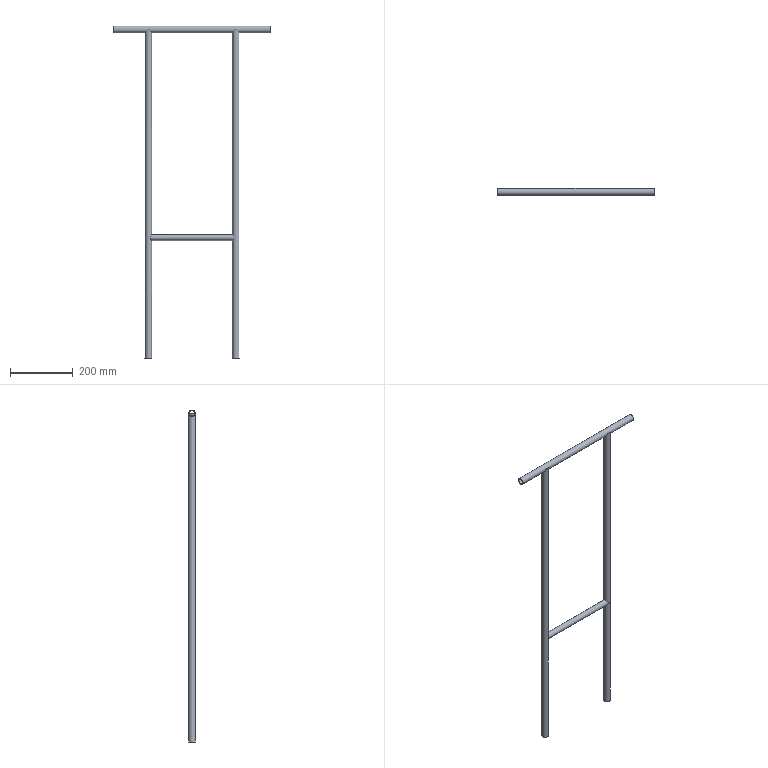Part | NX | features EXTRACT_DATUM_PLANE 4, DATUM_CSYS 3, SKETCH 3, EXTRUDE 2, Container 1, EXTRACT_BODY 1, Geometry Instance 1, MOVE_FACE 1, SWP104 1, UNITE 1 | 3 solids | 13 faces | box 500 x 21.5 x 1061 mm | volume 830822 mm3 | plane 7 | cylinder 6 | commonest cylinder face diameters 21.5 x3 10 x1 16.5 x1 18.964 x1
STEP:
#1=CARTESIAN_POINT('',(140.,6.69,378.039));
#2=VERTEX_POINT('',#1);
#3=CARTESIAN_POINT('',(140.,-0.01446,384.744));
#4=DIRECTION('',(1.,0.,0.));
#5=DIRECTION('',(0.,0.7071,-0.7071));
#6=AXIS2_PLACEMENT_3D('',#3,#4,#5);
#7=CIRCLE('',#6,9.482);
#8=EDGE_CURVE('',#2,#2,#7,.T.);
#9=ORIENTED_EDGE('',*,*,#8,.F.);
#10=EDGE_LOOP('',(#9));
#11=FACE_BOUND('',#10,.T.);
#12=CARTESIAN_POINT('',(-128.975,1.668,394.076));
#13=VERTEX_POINT('',#12);
#14=CARTESIAN_POINT('',(-130.069,5.387,392.822));
#15=CARTESIAN_POINT('',(-128.728,1.764,394.356));
#16=CARTESIAN_POINT('',(-128.865,-2.437,394.209));
#17=CARTESIAN_POINT('',(-130.39,-5.899,392.467));
#18=CARTESIAN_POINT('',(-132.147,-7.843,390.301));
#19=CARTESIAN_POINT('',(-133.504,-8.884,388.247));
#20=CARTESIAN_POINT('',(-134.376,-9.407,386.47));
#21=CARTESIAN_POINT('',(-134.691,-9.566,384.427));
#22=CARTESIAN_POINT('',(-134.144,-9.28,382.452));
#23=CARTESIAN_POINT('',(-133.204,-8.675,380.753));
#24=CARTESIAN_POINT('',(-131.813,-7.521,378.758));
#25=CARTESIAN_POINT('',(-130.099,-5.44,376.683));
#26=CARTESIAN_POINT('',(-128.737,-1.815,375.136));
#27=CARTESIAN_POINT('',(-128.853,2.381,375.272));
#28=CARTESIAN_POINT('',(-130.364,5.859,377.012));
#29=CARTESIAN_POINT('',(-132.111,7.81,379.177));
#30=CARTESIAN_POINT('',(-133.473,8.864,381.259));
#31=CARTESIAN_POINT('',(-134.334,9.383,383.043));
#32=CARTESIAN_POINT('',(-134.633,9.536,385.091));
#33=CARTESIAN_POINT('',(-134.084,9.245,387.059));
#34=CARTESIAN_POINT('',(-133.15,8.634,388.759));
#35=CARTESIAN_POINT('',(-131.774,7.48,390.745));
#36=CARTESIAN_POINT('',(-130.069,5.387,392.822));
#37=CARTESIAN_POINT('',(-128.728,1.764,394.356));
#38=CARTESIAN_POINT('',(-128.865,-2.437,394.209));
#39=B_SPLINE_CURVE_WITH_KNOTS('',3,(#14,#15,#16,#17,#18,#19,#20,#21,#22,#23,#24,#25,#26,#27,#28,#29,#30,#31,#32,#33,#34,#35,#36,#37,#38),.UNSPECIFIED.,.T.,.F.,(1,1,1,1,1,1,1,1,1,1,1,1,1,1,1,1,1,1,1,1,1,1,1,1,1,1,1,1,1),(-0.01005,-0.008036,-0.004018,0.,0.004018,0.008036,0.01205,0.01406,0.01607,0.01808,0.02009,0.0221,0.02411,0.02813,0.03214,0.03616,0.04018,0.0442,0.04621,0.04822,0.05023,0.05223,0.05424,0.05625,0.06027,0.06429,0.06831,0.07233,0.07634),.UNSPECIFIED.);
#40=EDGE_CURVE('',#13,#13,#39,.T.);
#41=ORIENTED_EDGE('',*,*,#40,.T.);
#42=EDGE_LOOP('',(#41));
#43=FACE_BOUND('',#42,.T.);
#44=CARTESIAN_POINT('',(-187.,-0.01446,384.744));
#45=DIRECTION('',(1.,0.,0.));
#46=DIRECTION('',(0.,0.,-1.));
#47=AXIS2_PLACEMENT_3D('',#44,#45,#46);
#48=CYLINDRICAL_SURFACE('',#47,9.482);
#49=ADVANCED_FACE('',(#11,#43),#48,.T.);
#50=ORIENTED_EDGE('',*,*,#8,.T.);
#51=EDGE_LOOP('',(#50));
#52=FACE_BOUND('',#51,.T.);
#53=CARTESIAN_POINT('',(140.,-0.01446,384.744));
#54=DIRECTION('',(1.,0.,0.));
#55=DIRECTION('',(0.,0.,-1.));
#56=AXIS2_PLACEMENT_3D('',#53,#54,#55);
#57=PLANE('',#56);
#58=ADVANCED_FACE('',(#52),#57,.T.);
#59=CARTESIAN_POINT('',(-139.595,-10.75,0.));
#60=VERTEX_POINT('',#59);
#61=CARTESIAN_POINT('',(-139.595,0.,0.));
#62=DIRECTION('',(0.,0.,1.));
#63=DIRECTION('',(0.,-1.,0.));
#64=AXIS2_PLACEMENT_3D('',#61,#62,#63);
#65=CIRCLE('',#64,10.75);
#66=EDGE_CURVE('',#60,#60,#65,.F.);
#67=ORIENTED_EDGE('',*,*,#66,.T.);
#68=EDGE_LOOP('',(#67));
#69=FACE_BOUND('',#68,.T.);
#70=CARTESIAN_POINT('',(-189.595,0.,0.));
#71=DIRECTION('',(0.,0.,1.));
#72=DIRECTION('',(-1.,0.,0.));
#73=AXIS2_PLACEMENT_3D('',#70,#71,#72);
#74=PLANE('',#73);
#75=ADVANCED_FACE('',(#69),#74,.F.);
#76=CARTESIAN_POINT('',(-139.595,-10.75,1050.));
#77=VERTEX_POINT('',#76);
#78=CARTESIAN_POINT('',(-139.595,0.,1050.));
#79=DIRECTION('',(0.,0.,-1.));
#80=DIRECTION('',(0.,-1.,0.));
#81=AXIS2_PLACEMENT_3D('',#78,#79,#80);
#82=CIRCLE('',#81,10.75);
#83=EDGE_CURVE('',#77,#77,#82,.F.);
#84=ORIENTED_EDGE('',*,*,#83,.T.);
#85=EDGE_LOOP('',(#84));
#86=FACE_BOUND('',#85,.T.);
#87=CARTESIAN_POINT('',(-189.595,0.,1050.));
#88=DIRECTION('',(0.,0.,1.));
#89=DIRECTION('',(-1.,0.,0.));
#90=AXIS2_PLACEMENT_3D('',#87,#88,#89);
#91=PLANE('',#90);
#92=ADVANCED_FACE('',(#86),#91,.T.);
#93=ORIENTED_EDGE('',*,*,#40,.F.);
#94=EDGE_LOOP('',(#93));
#95=FACE_BOUND('',#94,.T.);
#96=ORIENTED_EDGE('',*,*,#66,.F.);
#97=EDGE_LOOP('',(#96));
#98=FACE_BOUND('',#97,.T.);
#99=ORIENTED_EDGE('',*,*,#83,.F.);
#100=EDGE_LOOP('',(#99));
#101=FACE_BOUND('',#100,.T.);
#102=CARTESIAN_POINT('',(-139.595,0.,0.));
#103=DIRECTION('',(0.,0.,1.));
#104=DIRECTION('',(0.,-1.,0.));
#105=AXIS2_PLACEMENT_3D('',#102,#103,#104);
#106=CYLINDRICAL_SURFACE('',#105,10.75);
#107=ADVANCED_FACE('',(#95,#98,#101),#106,.T.);
#108=CLOSED_SHELL('',(#49,#58,#75,#92,#107));
#109=MANIFOLD_SOLID_BREP('',#108);
#110=CARTESIAN_POINT('',(140.,-10.75,0.));
#111=VERTEX_POINT('',#110);
#112=CARTESIAN_POINT('',(140.,0.,0.));
#113=DIRECTION('',(0.,0.,-1.));
#114=DIRECTION('',(0.,-1.,0.));
#115=AXIS2_PLACEMENT_3D('',#112,#113,#114);
#116=CIRCLE('',#115,10.75);
#117=EDGE_CURVE('',#111,#111,#116,.T.);
#118=ORIENTED_EDGE('',*,*,#117,.T.);
#119=EDGE_LOOP('',(#118));
#120=FACE_BOUND('',#119,.T.);
#121=CARTESIAN_POINT('',(140.,-5.,0.));
#122=VERTEX_POINT('',#121);
#123=CARTESIAN_POINT('',(140.,0.,0.));
#124=DIRECTION('',(0.,0.,1.));
#125=DIRECTION('',(0.,-1.,0.));
#126=AXIS2_PLACEMENT_3D('',#123,#124,#125);
#127=CIRCLE('',#126,5.);
#128=EDGE_CURVE('',#122,#122,#127,.F.);
#129=ORIENTED_EDGE('',*,*,#128,.F.);
#130=EDGE_LOOP('',(#129));
#131=FACE_BOUND('',#130,.T.);
#132=CARTESIAN_POINT('',(140.,0.,0.));
#133=DIRECTION('',(0.,0.,1.));
#134=DIRECTION('',(1.,0.,0.));
#135=AXIS2_PLACEMENT_3D('',#132,#133,#134);
#136=PLANE('',#135);
#137=ADVANCED_FACE('',(#120,#131),#136,.F.);
#138=CARTESIAN_POINT('',(140.,-5.,1050.));
#139=VERTEX_POINT('',#138);
#140=CARTESIAN_POINT('',(140.,0.,1050.));
#141=DIRECTION('',(0.,0.,1.));
#142=DIRECTION('',(0.,-1.,0.));
#143=AXIS2_PLACEMENT_3D('',#140,#141,#142);
#144=CIRCLE('',#143,5.);
#145=EDGE_CURVE('',#139,#139,#144,.T.);
#146=ORIENTED_EDGE('',*,*,#145,.F.);
#147=EDGE_LOOP('',(#146));
#148=FACE_BOUND('',#147,.T.);
#149=CARTESIAN_POINT('',(140.,-10.75,1050.));
#150=VERTEX_POINT('',#149);
#151=CARTESIAN_POINT('',(140.,0.,1050.));
#152=DIRECTION('',(0.,0.,1.));
#153=DIRECTION('',(0.,-1.,0.));
#154=AXIS2_PLACEMENT_3D('',#151,#152,#153);
#155=CIRCLE('',#154,10.75);
#156=EDGE_CURVE('',#150,#150,#155,.T.);
#157=ORIENTED_EDGE('',*,*,#156,.T.);
#158=EDGE_LOOP('',(#157));
#159=FACE_BOUND('',#158,.T.);
#160=CARTESIAN_POINT('',(140.,0.,1050.));
#161=DIRECTION('',(0.,0.,1.));
#162=DIRECTION('',(1.,0.,0.));
#163=AXIS2_PLACEMENT_3D('',#160,#161,#162);
#164=PLANE('',#163);
#165=ADVANCED_FACE('',(#148,#159),#164,.T.);
#166=ORIENTED_EDGE('',*,*,#117,.F.);
#167=EDGE_LOOP('',(#166));
#168=FACE_BOUND('',#167,.T.);
#169=ORIENTED_EDGE('',*,*,#156,.F.);
#170=EDGE_LOOP('',(#169));
#171=FACE_BOUND('',#170,.T.);
#172=CARTESIAN_POINT('',(140.,0.,0.));
#173=DIRECTION('',(0.,0.,1.));
#174=DIRECTION('',(0.,-1.,0.));
#175=AXIS2_PLACEMENT_3D('',#172,#173,#174);
#176=CYLINDRICAL_SURFACE('',#175,10.75);
#177=ADVANCED_FACE('',(#168,#171),#176,.T.);
#178=ORIENTED_EDGE('',*,*,#128,.T.);
#179=EDGE_LOOP('',(#178));
#180=FACE_BOUND('',#179,.T.);
#181=ORIENTED_EDGE('',*,*,#145,.T.);
#182=EDGE_LOOP('',(#181));
#183=FACE_BOUND('',#182,.T.);
#184=CARTESIAN_POINT('',(140.,0.,0.));
#185=DIRECTION('',(0.,0.,1.));
#186=DIRECTION('',(0.,-1.,0.));
#187=AXIS2_PLACEMENT_3D('',#184,#185,#186);
#188=CYLINDRICAL_SURFACE('',#187,5.);
#189=ADVANCED_FACE('',(#180,#183),#188,.F.);
#190=CLOSED_SHELL('',(#137,#165,#177,#189));
#191=MANIFOLD_SOLID_BREP('',#190);
#192=CARTESIAN_POINT('',(250.,0.,1060.75));
#193=VERTEX_POINT('',#192);
#194=CARTESIAN_POINT('',(250.,0.,1050.));
#195=DIRECTION('',(-1.,0.,0.));
#196=DIRECTION('',(0.,0.,1.));
#197=AXIS2_PLACEMENT_3D('',#194,#195,#196);
#198=CIRCLE('',#197,10.75);
#199=EDGE_CURVE('',#193,#193,#198,.T.);
#200=ORIENTED_EDGE('',*,*,#199,.T.);
#201=EDGE_LOOP('',(#200));
#202=FACE_BOUND('',#201,.T.);
#203=CARTESIAN_POINT('',(-250.,0.,1039.25));
#204=VERTEX_POINT('',#203);
#205=CARTESIAN_POINT('',(-250.,0.,1050.));
#206=DIRECTION('',(-1.,0.,0.));
#207=DIRECTION('',(0.,0.,-1.));
#208=AXIS2_PLACEMENT_3D('',#205,#206,#207);
#209=CIRCLE('',#208,10.75);
#210=EDGE_CURVE('',#204,#204,#209,.T.);
#211=ORIENTED_EDGE('',*,*,#210,.F.);
#212=EDGE_LOOP('',(#211));
#213=FACE_BOUND('',#212,.T.);
#214=CARTESIAN_POINT('',(-250.,0.,1050.));
#215=DIRECTION('',(1.,0.,0.));
#216=DIRECTION('',(0.,0.,-1.));
#217=AXIS2_PLACEMENT_3D('',#214,#215,#216);
#218=CYLINDRICAL_SURFACE('',#217,10.75);
#219=ADVANCED_FACE('',(#202,#213),#218,.T.);
#220=CARTESIAN_POINT('',(250.,0.,1058.25));
#221=VERTEX_POINT('',#220);
#222=CARTESIAN_POINT('',(250.,0.,1050.));
#223=DIRECTION('',(-1.,0.,0.));
#224=DIRECTION('',(0.,0.,1.));
#225=AXIS2_PLACEMENT_3D('',#222,#223,#224);
#226=CIRCLE('',#225,8.25);
#227=EDGE_CURVE('',#221,#221,#226,.T.);
#228=ORIENTED_EDGE('',*,*,#227,.F.);
#229=EDGE_LOOP('',(#228));
#230=FACE_BOUND('',#229,.T.);
#231=CARTESIAN_POINT('',(-250.,0.,1041.75));
#232=VERTEX_POINT('',#231);
#233=CARTESIAN_POINT('',(-250.,0.,1050.));
#234=DIRECTION('',(-1.,0.,0.));
#235=DIRECTION('',(0.,0.,-1.));
#236=AXIS2_PLACEMENT_3D('',#233,#234,#235);
#237=CIRCLE('',#236,8.25);
#238=EDGE_CURVE('',#232,#232,#237,.T.);
#239=ORIENTED_EDGE('',*,*,#238,.T.);
#240=EDGE_LOOP('',(#239));
#241=FACE_BOUND('',#240,.T.);
#242=CARTESIAN_POINT('',(-250.,0.,1050.));
#243=DIRECTION('',(1.,0.,0.));
#244=DIRECTION('',(0.,0.,-1.));
#245=AXIS2_PLACEMENT_3D('',#242,#243,#244);
#246=CYLINDRICAL_SURFACE('',#245,8.25);
#247=ADVANCED_FACE('',(#230,#241),#246,.F.);
#248=ORIENTED_EDGE('',*,*,#210,.T.);
#249=EDGE_LOOP('',(#248));
#250=FACE_BOUND('',#249,.T.);
#251=ORIENTED_EDGE('',*,*,#238,.F.);
#252=EDGE_LOOP('',(#251));
#253=FACE_BOUND('',#252,.T.);
#254=CARTESIAN_POINT('',(-250.,0.,1050.));
#255=DIRECTION('',(-1.,0.,0.));
#256=DIRECTION('',(0.,0.,1.));
#257=AXIS2_PLACEMENT_3D('',#254,#255,#256);
#258=PLANE('',#257);
#259=ADVANCED_FACE('',(#250,#253),#258,.T.);
#260=ORIENTED_EDGE('',*,*,#199,.F.);
#261=EDGE_LOOP('',(#260));
#262=FACE_BOUND('',#261,.T.);
#263=ORIENTED_EDGE('',*,*,#227,.T.);
#264=EDGE_LOOP('',(#263));
#265=FACE_BOUND('',#264,.T.);
#266=CARTESIAN_POINT('',(250.,0.,1050.));
#267=DIRECTION('',(-1.,0.,0.));
#268=DIRECTION('',(0.,0.,1.));
#269=AXIS2_PLACEMENT_3D('',#266,#267,#268);
#270=PLANE('',#269);
#271=ADVANCED_FACE('',(#262,#265),#270,.F.);
#272=CLOSED_SHELL('',(#219,#247,#259,#271));
#273=MANIFOLD_SOLID_BREP('',#272);
#274=(LENGTH_UNIT()NAMED_UNIT(*)SI_UNIT(.MILLI.,.METRE.));
#275=UNCERTAINTY_MEASURE_WITH_UNIT(LENGTH_MEASURE(0.0508),#274,'','');
#276=(NAMED_UNIT(*)PLANE_ANGLE_UNIT()SI_UNIT($,.RADIAN.));
#277=(NAMED_UNIT(*)SI_UNIT($,.STERADIAN.)SOLID_ANGLE_UNIT());
#278=(GEOMETRIC_REPRESENTATION_CONTEXT(3)GLOBAL_UNCERTAINTY_ASSIGNED_CONTEXT((#275))GLOBAL_UNIT_ASSIGNED_CONTEXT((#274,#276,#277))REPRESENTATION_CONTEXT('',''));
#279=ADVANCED_BREP_SHAPE_REPRESENTATION('',(#109,#191,#273),#278);